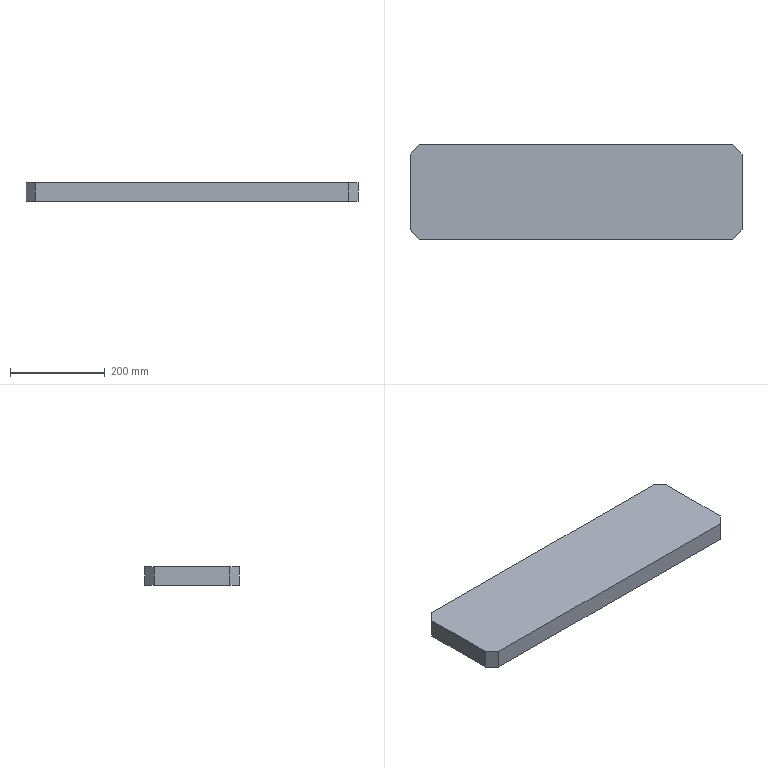Part | SolidWorks | features Chamfer 1, Extrusion 1 | 1 solid | 10 faces | box 700 x 200 x 40 mm | volume 5568000 mm3 | plane 10
STEP:
#1=CARTESIAN_POINT('',(350.,-80.,40.));
#2=VERTEX_POINT('',#1);
#3=CARTESIAN_POINT('',(350.,80.,40.));
#4=VERTEX_POINT('',#3);
#5=CARTESIAN_POINT('',(350.,100.,40.));
#6=DIRECTION('',(0.,1.,0.));
#7=VECTOR('',#6,1000.);
#8=LINE('',#5,#7);
#9=EDGE_CURVE('',#2,#4,#8,.T.);
#10=ORIENTED_EDGE('',*,*,#9,.F.);
#11=CARTESIAN_POINT('',(350.,-80.,0.));
#12=VERTEX_POINT('',#11);
#13=CARTESIAN_POINT('',(350.,-80.,40.));
#14=DIRECTION('',(0.,0.,-1.));
#15=VECTOR('',#14,1000.);
#16=LINE('',#13,#15);
#17=EDGE_CURVE('',#2,#12,#16,.T.);
#18=ORIENTED_EDGE('',*,*,#17,.T.);
#19=CARTESIAN_POINT('',(350.,80.,0.));
#20=VERTEX_POINT('',#19);
#21=CARTESIAN_POINT('',(350.,100.,0.));
#22=DIRECTION('',(0.,1.,0.));
#23=VECTOR('',#22,1000.);
#24=LINE('',#21,#23);
#25=EDGE_CURVE('',#12,#20,#24,.T.);
#26=ORIENTED_EDGE('',*,*,#25,.T.);
#27=CARTESIAN_POINT('',(350.,80.,40.));
#28=DIRECTION('',(0.,0.,1.));
#29=VECTOR('',#28,1000.);
#30=LINE('',#27,#29);
#31=EDGE_CURVE('',#20,#4,#30,.T.);
#32=ORIENTED_EDGE('',*,*,#31,.T.);
#33=EDGE_LOOP('',(#10,#18,#26,#32));
#34=FACE_OUTER_BOUND('',#33,.T.);
#35=CARTESIAN_POINT('',(350.,100.,40.));
#36=DIRECTION('',(-1.,0.,0.));
#37=DIRECTION('',(0.,0.,1.));
#38=AXIS2_PLACEMENT_3D('',#35,#36,#37);
#39=PLANE('',#38);
#40=ADVANCED_FACE('',(#34),#39,.F.);
#41=CARTESIAN_POINT('',(330.,100.,40.));
#42=VERTEX_POINT('',#41);
#43=CARTESIAN_POINT('',(-330.,100.,40.));
#44=VERTEX_POINT('',#43);
#45=CARTESIAN_POINT('',(-350.,100.,40.));
#46=DIRECTION('',(-1.,0.,0.));
#47=VECTOR('',#46,1000.);
#48=LINE('',#45,#47);
#49=EDGE_CURVE('',#42,#44,#48,.T.);
#50=ORIENTED_EDGE('',*,*,#49,.F.);
#51=CARTESIAN_POINT('',(330.,100.,0.));
#52=VERTEX_POINT('',#51);
#53=CARTESIAN_POINT('',(330.,100.,40.));
#54=DIRECTION('',(0.,0.,-1.));
#55=VECTOR('',#54,1000.);
#56=LINE('',#53,#55);
#57=EDGE_CURVE('',#42,#52,#56,.T.);
#58=ORIENTED_EDGE('',*,*,#57,.T.);
#59=CARTESIAN_POINT('',(-330.,100.,0.));
#60=VERTEX_POINT('',#59);
#61=CARTESIAN_POINT('',(-350.,100.,0.));
#62=DIRECTION('',(-1.,0.,0.));
#63=VECTOR('',#62,1000.);
#64=LINE('',#61,#63);
#65=EDGE_CURVE('',#52,#60,#64,.T.);
#66=ORIENTED_EDGE('',*,*,#65,.T.);
#67=CARTESIAN_POINT('',(-330.,100.,40.));
#68=DIRECTION('',(0.,0.,1.));
#69=VECTOR('',#68,1000.);
#70=LINE('',#67,#69);
#71=EDGE_CURVE('',#60,#44,#70,.T.);
#72=ORIENTED_EDGE('',*,*,#71,.T.);
#73=EDGE_LOOP('',(#50,#58,#66,#72));
#74=FACE_OUTER_BOUND('',#73,.T.);
#75=CARTESIAN_POINT('',(-350.,100.,40.));
#76=DIRECTION('',(0.,-1.,0.));
#77=DIRECTION('',(0.,0.,-1.));
#78=AXIS2_PLACEMENT_3D('',#75,#76,#77);
#79=PLANE('',#78);
#80=ADVANCED_FACE('',(#74),#79,.F.);
#81=CARTESIAN_POINT('',(-350.,80.,0.));
#82=VERTEX_POINT('',#81);
#83=CARTESIAN_POINT('',(-350.,-80.,0.));
#84=VERTEX_POINT('',#83);
#85=CARTESIAN_POINT('',(-350.,100.,0.));
#86=DIRECTION('',(0.,-1.,0.));
#87=VECTOR('',#86,1000.);
#88=LINE('',#85,#87);
#89=EDGE_CURVE('',#82,#84,#88,.T.);
#90=ORIENTED_EDGE('',*,*,#89,.T.);
#91=CARTESIAN_POINT('',(-350.,-80.,40.));
#92=VERTEX_POINT('',#91);
#93=CARTESIAN_POINT('',(-350.,-80.,40.));
#94=DIRECTION('',(0.,0.,1.));
#95=VECTOR('',#94,1000.);
#96=LINE('',#93,#95);
#97=EDGE_CURVE('',#84,#92,#96,.T.);
#98=ORIENTED_EDGE('',*,*,#97,.T.);
#99=CARTESIAN_POINT('',(-350.,80.,40.));
#100=VERTEX_POINT('',#99);
#101=CARTESIAN_POINT('',(-350.,100.,40.));
#102=DIRECTION('',(0.,-1.,0.));
#103=VECTOR('',#102,1000.);
#104=LINE('',#101,#103);
#105=EDGE_CURVE('',#100,#92,#104,.T.);
#106=ORIENTED_EDGE('',*,*,#105,.F.);
#107=CARTESIAN_POINT('',(-350.,80.,40.));
#108=DIRECTION('',(0.,0.,-1.));
#109=VECTOR('',#108,1000.);
#110=LINE('',#107,#109);
#111=EDGE_CURVE('',#100,#82,#110,.T.);
#112=ORIENTED_EDGE('',*,*,#111,.T.);
#113=EDGE_LOOP('',(#90,#98,#106,#112));
#114=FACE_OUTER_BOUND('',#113,.T.);
#115=CARTESIAN_POINT('',(-350.,100.,40.));
#116=DIRECTION('',(1.,0.,0.));
#117=DIRECTION('',(0.,0.,-1.));
#118=AXIS2_PLACEMENT_3D('',#115,#116,#117);
#119=PLANE('',#118);
#120=ADVANCED_FACE('',(#114),#119,.F.);
#121=CARTESIAN_POINT('',(-330.,-100.,0.));
#122=VERTEX_POINT('',#121);
#123=CARTESIAN_POINT('',(330.,-100.,0.));
#124=VERTEX_POINT('',#123);
#125=CARTESIAN_POINT('',(-350.,-100.,0.));
#126=DIRECTION('',(1.,0.,0.));
#127=VECTOR('',#126,1000.);
#128=LINE('',#125,#127);
#129=EDGE_CURVE('',#122,#124,#128,.T.);
#130=ORIENTED_EDGE('',*,*,#129,.T.);
#131=CARTESIAN_POINT('',(330.,-100.,40.));
#132=VERTEX_POINT('',#131);
#133=CARTESIAN_POINT('',(330.,-100.,40.));
#134=DIRECTION('',(0.,0.,1.));
#135=VECTOR('',#134,1000.);
#136=LINE('',#133,#135);
#137=EDGE_CURVE('',#124,#132,#136,.T.);
#138=ORIENTED_EDGE('',*,*,#137,.T.);
#139=CARTESIAN_POINT('',(-330.,-100.,40.));
#140=VERTEX_POINT('',#139);
#141=CARTESIAN_POINT('',(-350.,-100.,40.));
#142=DIRECTION('',(1.,0.,0.));
#143=VECTOR('',#142,1000.);
#144=LINE('',#141,#143);
#145=EDGE_CURVE('',#140,#132,#144,.T.);
#146=ORIENTED_EDGE('',*,*,#145,.F.);
#147=CARTESIAN_POINT('',(-330.,-100.,40.));
#148=DIRECTION('',(0.,0.,-1.));
#149=VECTOR('',#148,1000.);
#150=LINE('',#147,#149);
#151=EDGE_CURVE('',#140,#122,#150,.T.);
#152=ORIENTED_EDGE('',*,*,#151,.T.);
#153=EDGE_LOOP('',(#130,#138,#146,#152));
#154=FACE_OUTER_BOUND('',#153,.T.);
#155=CARTESIAN_POINT('',(-350.,-100.,40.));
#156=DIRECTION('',(0.,1.,0.));
#157=DIRECTION('',(0.,0.,1.));
#158=AXIS2_PLACEMENT_3D('',#155,#156,#157);
#159=PLANE('',#158);
#160=ADVANCED_FACE('',(#154),#159,.F.);
#161=ORIENTED_EDGE('',*,*,#145,.T.);
#162=CARTESIAN_POINT('',(215.,-215.,40.));
#163=DIRECTION('',(0.7071,0.7071,0.));
#164=VECTOR('',#163,1000.);
#165=LINE('',#162,#164);
#166=EDGE_CURVE('',#132,#2,#165,.T.);
#167=ORIENTED_EDGE('',*,*,#166,.T.);
#168=ORIENTED_EDGE('',*,*,#9,.T.);
#169=CARTESIAN_POINT('',(215.,215.,40.));
#170=DIRECTION('',(-0.7071,0.7071,0.));
#171=VECTOR('',#170,1000.);
#172=LINE('',#169,#171);
#173=EDGE_CURVE('',#4,#42,#172,.T.);
#174=ORIENTED_EDGE('',*,*,#173,.T.);
#175=ORIENTED_EDGE('',*,*,#49,.T.);
#176=CARTESIAN_POINT('',(-215.,215.,40.));
#177=DIRECTION('',(-0.7071,-0.7071,0.));
#178=VECTOR('',#177,1000.);
#179=LINE('',#176,#178);
#180=EDGE_CURVE('',#44,#100,#179,.T.);
#181=ORIENTED_EDGE('',*,*,#180,.T.);
#182=ORIENTED_EDGE('',*,*,#105,.T.);
#183=CARTESIAN_POINT('',(-215.,-215.,40.));
#184=DIRECTION('',(0.7071,-0.7071,0.));
#185=VECTOR('',#184,1000.);
#186=LINE('',#183,#185);
#187=EDGE_CURVE('',#92,#140,#186,.T.);
#188=ORIENTED_EDGE('',*,*,#187,.T.);
#189=EDGE_LOOP('',(#161,#167,#168,#174,#175,#181,#182,#188));
#190=FACE_OUTER_BOUND('',#189,.T.);
#191=CARTESIAN_POINT('',(0.,0.,40.));
#192=DIRECTION('',(0.,0.,1.));
#193=DIRECTION('',(1.,0.,0.));
#194=AXIS2_PLACEMENT_3D('',#191,#192,#193);
#195=PLANE('',#194);
#196=ADVANCED_FACE('',(#190),#195,.T.);
#197=ORIENTED_EDGE('',*,*,#25,.F.);
#198=CARTESIAN_POINT('',(350.,-80.,0.));
#199=DIRECTION('',(-0.7071,-0.7071,0.));
#200=VECTOR('',#199,1000.);
#201=LINE('',#198,#200);
#202=EDGE_CURVE('',#12,#124,#201,.T.);
#203=ORIENTED_EDGE('',*,*,#202,.T.);
#204=ORIENTED_EDGE('',*,*,#129,.F.);
#205=CARTESIAN_POINT('',(-330.,-100.,0.));
#206=DIRECTION('',(-0.7071,0.7071,0.));
#207=VECTOR('',#206,1000.);
#208=LINE('',#205,#207);
#209=EDGE_CURVE('',#122,#84,#208,.T.);
#210=ORIENTED_EDGE('',*,*,#209,.T.);
#211=ORIENTED_EDGE('',*,*,#89,.F.);
#212=CARTESIAN_POINT('',(-350.,80.,0.));
#213=DIRECTION('',(0.7071,0.7071,0.));
#214=VECTOR('',#213,1000.);
#215=LINE('',#212,#214);
#216=EDGE_CURVE('',#82,#60,#215,.T.);
#217=ORIENTED_EDGE('',*,*,#216,.T.);
#218=ORIENTED_EDGE('',*,*,#65,.F.);
#219=CARTESIAN_POINT('',(330.,100.,0.));
#220=DIRECTION('',(0.7071,-0.7071,0.));
#221=VECTOR('',#220,1000.);
#222=LINE('',#219,#221);
#223=EDGE_CURVE('',#52,#20,#222,.T.);
#224=ORIENTED_EDGE('',*,*,#223,.T.);
#225=EDGE_LOOP('',(#197,#203,#204,#210,#211,#217,#218,#224));
#226=FACE_OUTER_BOUND('',#225,.T.);
#227=CARTESIAN_POINT('',(0.,0.,0.));
#228=DIRECTION('',(0.,0.,1.));
#229=DIRECTION('',(1.,0.,0.));
#230=AXIS2_PLACEMENT_3D('',#227,#228,#229);
#231=PLANE('',#230);
#232=ADVANCED_FACE('',(#226),#231,.F.);
#233=ORIENTED_EDGE('',*,*,#166,.F.);
#234=ORIENTED_EDGE('',*,*,#137,.F.);
#235=ORIENTED_EDGE('',*,*,#202,.F.);
#236=ORIENTED_EDGE('',*,*,#17,.F.);
#237=EDGE_LOOP('',(#233,#234,#235,#236));
#238=FACE_OUTER_BOUND('',#237,.T.);
#239=CARTESIAN_POINT('',(350.,-80.,40.));
#240=DIRECTION('',(-0.7071,0.7071,0.));
#241=DIRECTION('',(0.,0.,-1.));
#242=AXIS2_PLACEMENT_3D('',#239,#240,#241);
#243=PLANE('',#242);
#244=ADVANCED_FACE('',(#238),#243,.F.);
#245=ORIENTED_EDGE('',*,*,#173,.F.);
#246=ORIENTED_EDGE('',*,*,#31,.F.);
#247=ORIENTED_EDGE('',*,*,#223,.F.);
#248=ORIENTED_EDGE('',*,*,#57,.F.);
#249=EDGE_LOOP('',(#245,#246,#247,#248));
#250=FACE_OUTER_BOUND('',#249,.T.);
#251=CARTESIAN_POINT('',(330.,100.,40.));
#252=DIRECTION('',(-0.7071,-0.7071,0.));
#253=DIRECTION('',(0.,0.,-1.));
#254=AXIS2_PLACEMENT_3D('',#251,#252,#253);
#255=PLANE('',#254);
#256=ADVANCED_FACE('',(#250),#255,.F.);
#257=ORIENTED_EDGE('',*,*,#187,.F.);
#258=ORIENTED_EDGE('',*,*,#97,.F.);
#259=ORIENTED_EDGE('',*,*,#209,.F.);
#260=ORIENTED_EDGE('',*,*,#151,.F.);
#261=EDGE_LOOP('',(#257,#258,#259,#260));
#262=FACE_OUTER_BOUND('',#261,.T.);
#263=CARTESIAN_POINT('',(-330.,-100.,40.));
#264=DIRECTION('',(0.7071,0.7071,0.));
#265=DIRECTION('',(0.,0.,-1.));
#266=AXIS2_PLACEMENT_3D('',#263,#264,#265);
#267=PLANE('',#266);
#268=ADVANCED_FACE('',(#262),#267,.F.);
#269=ORIENTED_EDGE('',*,*,#180,.F.);
#270=ORIENTED_EDGE('',*,*,#71,.F.);
#271=ORIENTED_EDGE('',*,*,#216,.F.);
#272=ORIENTED_EDGE('',*,*,#111,.F.);
#273=EDGE_LOOP('',(#269,#270,#271,#272));
#274=FACE_OUTER_BOUND('',#273,.T.);
#275=CARTESIAN_POINT('',(-350.,80.,40.));
#276=DIRECTION('',(0.7071,-0.7071,0.));
#277=DIRECTION('',(0.,0.,-1.));
#278=AXIS2_PLACEMENT_3D('',#275,#276,#277);
#279=PLANE('',#278);
#280=ADVANCED_FACE('',(#274),#279,.F.);
#281=CLOSED_SHELL('',(#40,#80,#120,#160,#196,#232,#244,#256,#268,#280));
#282=MANIFOLD_SOLID_BREP('',#281);
#283=CARTESIAN_POINT('',(0.,0.,0.));
#284=DIRECTION('',(0.,0.,1.));
#285=DIRECTION('',(1.,0.,0.));
#286=AXIS2_PLACEMENT_3D('',#283,#284,#285);
#287=(LENGTH_UNIT()NAMED_UNIT(*)SI_UNIT(.MILLI.,.METRE.));
#288=UNCERTAINTY_MEASURE_WITH_UNIT(LENGTH_MEASURE(0.00001),#287,'','');
#289=(NAMED_UNIT(*)PLANE_ANGLE_UNIT()SI_UNIT($,.RADIAN.));
#290=(NAMED_UNIT(*)SI_UNIT($,.STERADIAN.)SOLID_ANGLE_UNIT());
#291=(GEOMETRIC_REPRESENTATION_CONTEXT(3)GLOBAL_UNCERTAINTY_ASSIGNED_CONTEXT((#288))GLOBAL_UNIT_ASSIGNED_CONTEXT((#287,#289,#290))REPRESENTATION_CONTEXT('',''));
#292=ADVANCED_BREP_SHAPE_REPRESENTATION('',(#282,#286),#291);